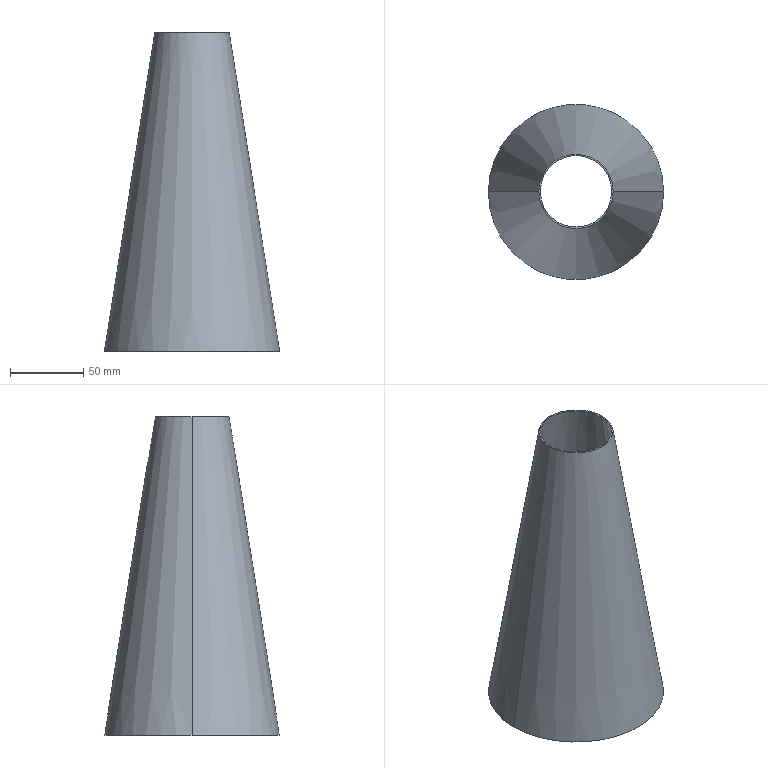Part | SolidWorks | features BaseBody 1 | 1 solid | 6 faces | box 120 x 120 x 218 mm | volume 58583 mm3 | cone 4 | plane 2
STEP:
#1=CARTESIAN_POINT('',(24.488,0.,218.));
#2=VERTEX_POINT('',#1);
#3=CARTESIAN_POINT('',(58.988,0.,0.));
#4=VERTEX_POINT('',#3);
#5=CARTESIAN_POINT('',(24.512,0.,217.844));
#6=DIRECTION('',(0.1563,0.,-0.9877));
#7=VECTOR('',#6,1000.);
#8=LINE('',#5,#7);
#9=EDGE_CURVE('',#2,#4,#8,.T.);
#10=ORIENTED_EDGE('',*,*,#9,.F.);
#11=CARTESIAN_POINT('',(-24.488,0.,218.));
#12=VERTEX_POINT('',#11);
#13=CARTESIAN_POINT('',(0.,0.,218.));
#14=DIRECTION('',(0.,0.,1.));
#15=DIRECTION('',(1.,0.,0.));
#16=AXIS2_PLACEMENT_3D('',#13,#14,#15);
#17=CIRCLE('',#16,24.488);
#18=EDGE_CURVE('',#2,#12,#17,.T.);
#19=ORIENTED_EDGE('',*,*,#18,.T.);
#20=CARTESIAN_POINT('',(-58.988,0.,0.));
#21=VERTEX_POINT('',#20);
#22=CARTESIAN_POINT('',(-24.512,0.,217.844));
#23=DIRECTION('',(-0.1563,0.,-0.9877));
#24=VECTOR('',#23,1000.);
#25=LINE('',#22,#24);
#26=EDGE_CURVE('',#12,#21,#25,.T.);
#27=ORIENTED_EDGE('',*,*,#26,.T.);
#28=CARTESIAN_POINT('',(0.,0.,0.));
#29=DIRECTION('',(0.,0.,1.));
#30=DIRECTION('',(1.,0.,0.));
#31=AXIS2_PLACEMENT_3D('',#28,#29,#30);
#32=CIRCLE('',#31,58.988);
#33=EDGE_CURVE('',#4,#21,#32,.T.);
#34=ORIENTED_EDGE('',*,*,#33,.F.);
#35=EDGE_LOOP('',(#10,#19,#27,#34));
#36=FACE_OUTER_BOUND('',#35,.T.);
#37=CARTESIAN_POINT('',(0.,0.,217.844));
#38=DIRECTION('',(0.,0.,-1.));
#39=DIRECTION('',(-1.,0.,0.));
#40=AXIS2_PLACEMENT_3D('',#37,#38,#39);
#41=CONICAL_SURFACE('',#40,24.512,0.157);
#42=ADVANCED_FACE('',(#36),#41,.F.);
#43=CARTESIAN_POINT('',(25.5,0.,218.));
#44=VERTEX_POINT('',#43);
#45=CARTESIAN_POINT('',(60.,0.,0.));
#46=VERTEX_POINT('',#45);
#47=CARTESIAN_POINT('',(25.5,0.,218.));
#48=DIRECTION('',(0.1563,0.,-0.9877));
#49=VECTOR('',#48,1000.);
#50=LINE('',#47,#49);
#51=EDGE_CURVE('',#44,#46,#50,.T.);
#52=ORIENTED_EDGE('',*,*,#51,.F.);
#53=CARTESIAN_POINT('',(-25.5,0.,218.));
#54=VERTEX_POINT('',#53);
#55=CARTESIAN_POINT('',(0.,0.,218.));
#56=DIRECTION('',(0.,0.,1.));
#57=DIRECTION('',(1.,0.,0.));
#58=AXIS2_PLACEMENT_3D('',#55,#56,#57);
#59=CIRCLE('',#58,25.5);
#60=EDGE_CURVE('',#54,#44,#59,.T.);
#61=ORIENTED_EDGE('',*,*,#60,.F.);
#62=CARTESIAN_POINT('',(-60.,0.,0.));
#63=VERTEX_POINT('',#62);
#64=CARTESIAN_POINT('',(-25.5,0.,218.));
#65=DIRECTION('',(-0.1563,0.,-0.9877));
#66=VECTOR('',#65,1000.);
#67=LINE('',#64,#66);
#68=EDGE_CURVE('',#54,#63,#67,.T.);
#69=ORIENTED_EDGE('',*,*,#68,.T.);
#70=CARTESIAN_POINT('',(0.,0.,0.));
#71=DIRECTION('',(0.,0.,1.));
#72=DIRECTION('',(1.,0.,0.));
#73=AXIS2_PLACEMENT_3D('',#70,#71,#72);
#74=CIRCLE('',#73,60.);
#75=EDGE_CURVE('',#63,#46,#74,.T.);
#76=ORIENTED_EDGE('',*,*,#75,.T.);
#77=EDGE_LOOP('',(#52,#61,#69,#76));
#78=FACE_OUTER_BOUND('',#77,.T.);
#79=CARTESIAN_POINT('',(0.,0.,218.));
#80=DIRECTION('',(0.,0.,-1.));
#81=DIRECTION('',(-1.,0.,0.));
#82=AXIS2_PLACEMENT_3D('',#79,#80,#81);
#83=CONICAL_SURFACE('',#82,25.5,0.157);
#84=ADVANCED_FACE('',(#78),#83,.T.);
#85=CARTESIAN_POINT('',(0.,0.,218.));
#86=DIRECTION('',(0.,0.,1.));
#87=DIRECTION('',(1.,0.,0.));
#88=AXIS2_PLACEMENT_3D('',#85,#86,#87);
#89=CIRCLE('',#88,24.488);
#90=EDGE_CURVE('',#12,#2,#89,.T.);
#91=ORIENTED_EDGE('',*,*,#90,.F.);
#92=ORIENTED_EDGE('',*,*,#18,.F.);
#93=EDGE_LOOP('',(#91,#92));
#94=FACE_BOUND('',#93,.T.);
#95=ORIENTED_EDGE('',*,*,#60,.T.);
#96=CARTESIAN_POINT('',(0.,0.,218.));
#97=DIRECTION('',(0.,0.,1.));
#98=DIRECTION('',(1.,0.,0.));
#99=AXIS2_PLACEMENT_3D('',#96,#97,#98);
#100=CIRCLE('',#99,25.5);
#101=EDGE_CURVE('',#44,#54,#100,.T.);
#102=ORIENTED_EDGE('',*,*,#101,.T.);
#103=EDGE_LOOP('',(#95,#102));
#104=FACE_OUTER_BOUND('',#103,.T.);
#105=CARTESIAN_POINT('',(0.,0.,218.));
#106=DIRECTION('',(0.,0.,1.));
#107=DIRECTION('',(1.,0.,0.));
#108=AXIS2_PLACEMENT_3D('',#105,#106,#107);
#109=PLANE('',#108);
#110=ADVANCED_FACE('',(#94,#104),#109,.T.);
#111=CARTESIAN_POINT('',(0.,0.,0.));
#112=DIRECTION('',(0.,0.,1.));
#113=DIRECTION('',(1.,0.,0.));
#114=AXIS2_PLACEMENT_3D('',#111,#112,#113);
#115=CIRCLE('',#114,58.988);
#116=EDGE_CURVE('',#21,#4,#115,.T.);
#117=ORIENTED_EDGE('',*,*,#116,.T.);
#118=ORIENTED_EDGE('',*,*,#33,.T.);
#119=EDGE_LOOP('',(#117,#118));
#120=FACE_BOUND('',#119,.T.);
#121=ORIENTED_EDGE('',*,*,#75,.F.);
#122=CARTESIAN_POINT('',(0.,0.,0.));
#123=DIRECTION('',(0.,0.,1.));
#124=DIRECTION('',(1.,0.,0.));
#125=AXIS2_PLACEMENT_3D('',#122,#123,#124);
#126=CIRCLE('',#125,60.);
#127=EDGE_CURVE('',#46,#63,#126,.T.);
#128=ORIENTED_EDGE('',*,*,#127,.F.);
#129=EDGE_LOOP('',(#121,#128));
#130=FACE_OUTER_BOUND('',#129,.T.);
#131=CARTESIAN_POINT('',(0.,0.,0.));
#132=DIRECTION('',(0.,0.,1.));
#133=DIRECTION('',(1.,0.,0.));
#134=AXIS2_PLACEMENT_3D('',#131,#132,#133);
#135=PLANE('',#134);
#136=ADVANCED_FACE('',(#120,#130),#135,.F.);
#137=ORIENTED_EDGE('',*,*,#101,.F.);
#138=ORIENTED_EDGE('',*,*,#51,.T.);
#139=ORIENTED_EDGE('',*,*,#127,.T.);
#140=ORIENTED_EDGE('',*,*,#68,.F.);
#141=EDGE_LOOP('',(#137,#138,#139,#140));
#142=FACE_OUTER_BOUND('',#141,.T.);
#143=CARTESIAN_POINT('',(0.,0.,218.));
#144=DIRECTION('',(0.,0.,-1.));
#145=DIRECTION('',(-1.,0.,0.));
#146=AXIS2_PLACEMENT_3D('',#143,#144,#145);
#147=CONICAL_SURFACE('',#146,25.5,0.157);
#148=ADVANCED_FACE('',(#142),#147,.T.);
#149=ORIENTED_EDGE('',*,*,#90,.T.);
#150=ORIENTED_EDGE('',*,*,#9,.T.);
#151=ORIENTED_EDGE('',*,*,#116,.F.);
#152=ORIENTED_EDGE('',*,*,#26,.F.);
#153=EDGE_LOOP('',(#149,#150,#151,#152));
#154=FACE_OUTER_BOUND('',#153,.T.);
#155=CARTESIAN_POINT('',(0.,0.,217.844));
#156=DIRECTION('',(0.,0.,-1.));
#157=DIRECTION('',(-1.,0.,0.));
#158=AXIS2_PLACEMENT_3D('',#155,#156,#157);
#159=CONICAL_SURFACE('',#158,24.512,0.157);
#160=ADVANCED_FACE('',(#154),#159,.F.);
#161=CLOSED_SHELL('',(#42,#84,#110,#136,#148,#160));
#162=MANIFOLD_SOLID_BREP('',#161);
#163=CARTESIAN_POINT('',(0.,0.,0.));
#164=DIRECTION('',(0.,0.,1.));
#165=DIRECTION('',(1.,0.,0.));
#166=AXIS2_PLACEMENT_3D('',#163,#164,#165);
#167=(LENGTH_UNIT()NAMED_UNIT(*)SI_UNIT(.MILLI.,.METRE.));
#168=UNCERTAINTY_MEASURE_WITH_UNIT(LENGTH_MEASURE(0.00001),#167,'','');
#169=(NAMED_UNIT(*)PLANE_ANGLE_UNIT()SI_UNIT($,.RADIAN.));
#170=(NAMED_UNIT(*)SI_UNIT($,.STERADIAN.)SOLID_ANGLE_UNIT());
#171=(GEOMETRIC_REPRESENTATION_CONTEXT(3)GLOBAL_UNCERTAINTY_ASSIGNED_CONTEXT((#168))GLOBAL_UNIT_ASSIGNED_CONTEXT((#167,#169,#170))REPRESENTATION_CONTEXT('',''));
#172=ADVANCED_BREP_SHAPE_REPRESENTATION('',(#162,#166),#171);